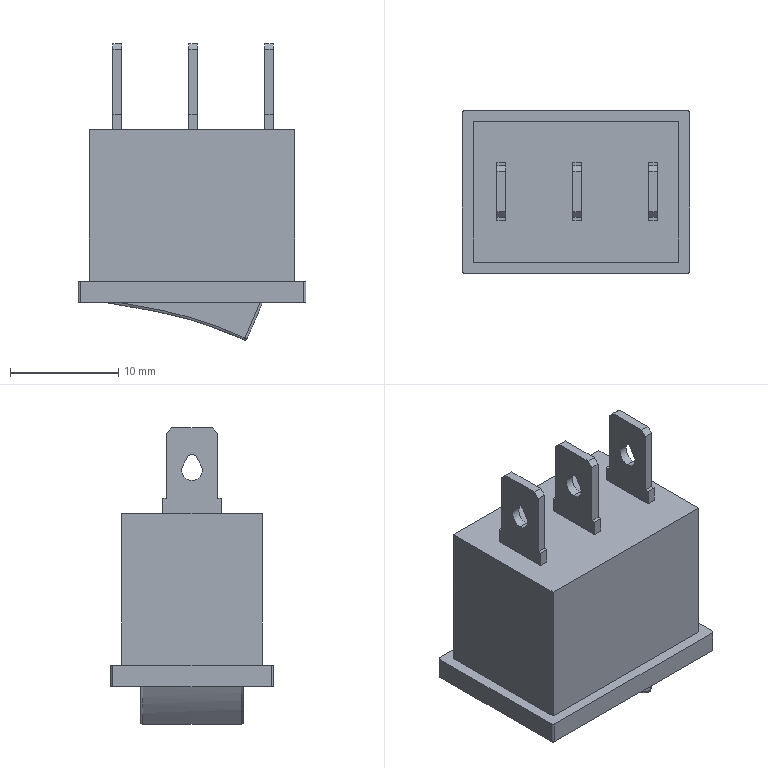Part | STEP file | three-pin two-speed power switch KCD4-16A-250 | 1 solid | 75 faces | box 21 x 15 x 27.336 mm | volume 4367 mm3 | plane 53 | cylinder 17 | spline 3 | sphere 2 | commonest cylinder face diameters 0.4 x8 1.9 x6 0.9 x3